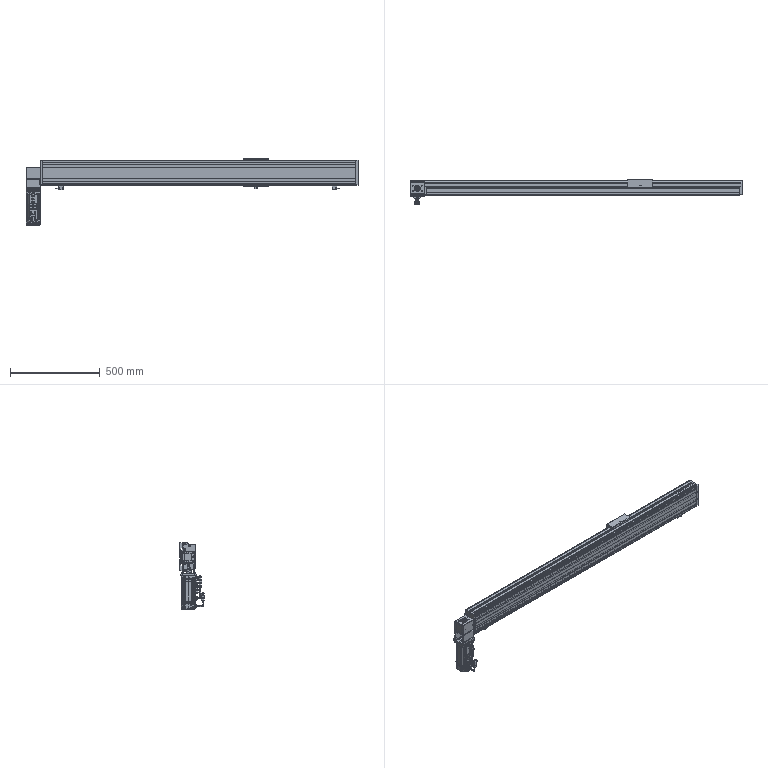Part | NX | features BREP 122 | 97 solids | 4761 faces | volume 6731601 mm3 | plane 2275 | cylinder 1529 | cone 559 | torus 207 | spline 124 | sphere 67 | commonest cylinder face diameters 2 x156 1 x125 3 x115 5 x70 10 x68 2.5 x62